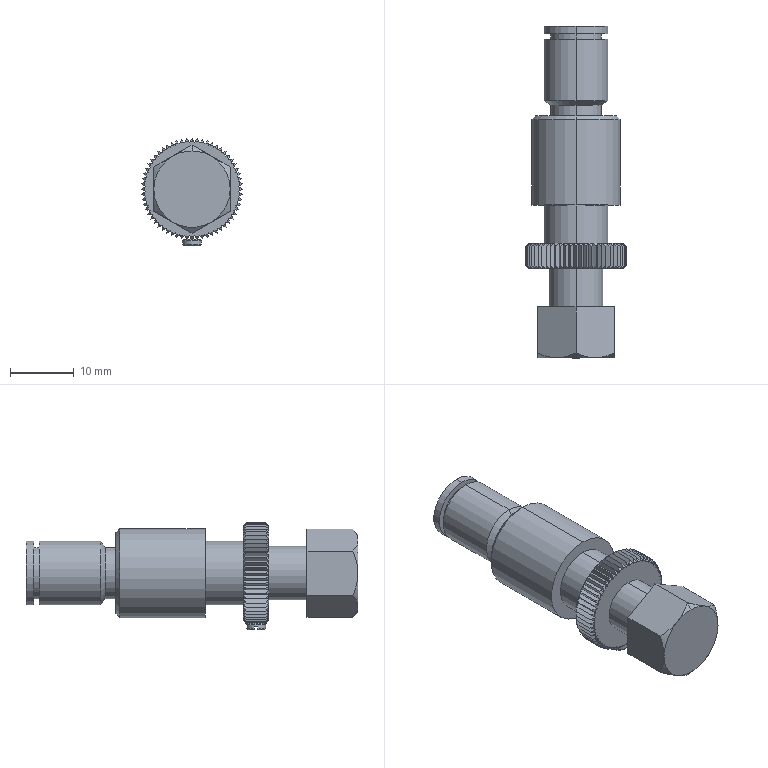Part | STEP file | _J-WES26-d10-001 | 1 solid | 300 faces | box 16 x 52.1 x 16.9 mm | volume 5380 mm3 | plane 145 | cone 137 | cylinder 18 | commonest cylinder face diameters 10 x6 8 x4 3 x2 6 x2 8.4 x2 14 x2